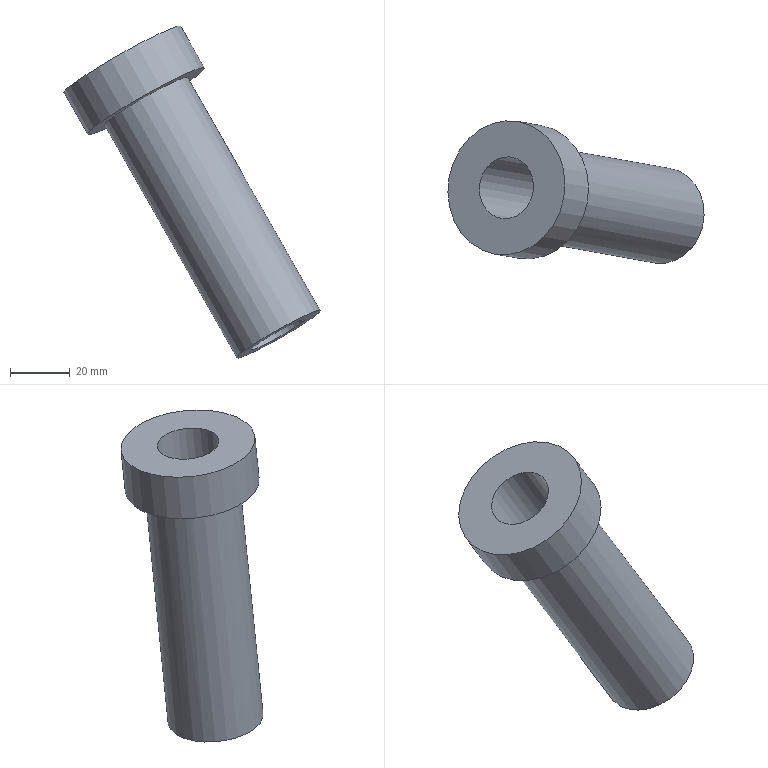Part | NX | features solid 2 | 1 solid | 6 faces | box 85.704 x 47.558 x 111.049 mm | volume 61811 mm3 | cylinder 3 | plane 3 | commonest cylinder face diameters 20.8 x1 32 x1 45 x1
STEP:
#1=CARTESIAN_POINT('',(-987.93,513.799,94.306));
#2=VERTEX_POINT('',#1);
#3=CARTESIAN_POINT('',(-996.8,515.363,89.106));
#4=DIRECTION('',(0.4924,-0.08682,-0.866));
#5=DIRECTION('',(0.8529,-0.1504,0.5));
#6=AXIS2_PLACEMENT_3D('',#3,#4,#5);
#7=CIRCLE('',#6,10.4);
#8=EDGE_CURVE('',#2,#2,#7,.T.);
#9=ORIENTED_EDGE('',*,*,#8,.F.);
#10=EDGE_LOOP('',(#9));
#11=FACE_BOUND('',#10,.T.);
#12=CARTESIAN_POINT('',(-953.646,506.16,-7.834));
#13=VERTEX_POINT('',#12);
#14=CARTESIAN_POINT('',(-944.605,506.16,-2.693));
#15=DIRECTION('',(0.4924,-0.08682,-0.866));
#16=DIRECTION('',(-0.8693,0.,-0.4943));
#17=AXIS2_PLACEMENT_3D('',#14,#15,#16);
#18=CIRCLE('',#17,10.4);
#19=EDGE_CURVE('',#13,#13,#18,.T.);
#20=ORIENTED_EDGE('',*,*,#19,.T.);
#21=EDGE_LOOP('',(#20));
#22=FACE_BOUND('',#21,.T.);
#23=CARTESIAN_POINT('',(-1026.345,520.573,141.067));
#24=DIRECTION('',(0.4924,-0.08682,-0.866));
#25=DIRECTION('',(-0.1736,-0.9848,0.));
#26=AXIS2_PLACEMENT_3D('',#23,#24,#25);
#27=CYLINDRICAL_SURFACE('',#26,10.4);
#28=ADVANCED_FACE('',(#11,#22),#27,.F.);
#29=CARTESIAN_POINT('',(-1002.568,516.38,67.249));
#30=VERTEX_POINT('',#29);
#31=CARTESIAN_POINT('',(-988.922,513.974,75.249));
#32=DIRECTION('',(-0.4924,0.08682,0.866));
#33=DIRECTION('',(-0.8529,0.1504,-0.5));
#34=AXIS2_PLACEMENT_3D('',#31,#32,#33);
#35=CIRCLE('',#34,16.);
#36=EDGE_CURVE('',#30,#30,#35,.T.);
#37=ORIENTED_EDGE('',*,*,#36,.F.);
#38=EDGE_LOOP('',(#37));
#39=FACE_BOUND('',#38,.T.);
#40=CARTESIAN_POINT('',(-958.514,506.16,-10.601));
#41=VERTEX_POINT('',#40);
#42=CARTESIAN_POINT('',(-944.605,506.16,-2.693));
#43=DIRECTION('',(0.4924,-0.08682,-0.866));
#44=DIRECTION('',(-0.8693,0.,-0.4943));
#45=AXIS2_PLACEMENT_3D('',#42,#43,#44);
#46=CIRCLE('',#45,16.);
#47=EDGE_CURVE('',#41,#41,#46,.T.);
#48=ORIENTED_EDGE('',*,*,#47,.F.);
#49=EDGE_LOOP('',(#48));
#50=FACE_BOUND('',#49,.T.);
#51=CARTESIAN_POINT('',(-1018.466,519.184,127.211));
#52=DIRECTION('',(0.4924,-0.08682,-0.866));
#53=DIRECTION('',(-0.1736,-0.9848,0.));
#54=AXIS2_PLACEMENT_3D('',#51,#52,#53);
#55=CYLINDRICAL_SURFACE('',#54,16.);
#56=ADVANCED_FACE('',(#39,#50),#55,.T.);
#57=CARTESIAN_POINT('',(-1008.111,517.358,63.999));
#58=VERTEX_POINT('',#57);
#59=CARTESIAN_POINT('',(-988.922,513.974,75.249));
#60=DIRECTION('',(-0.4924,0.08682,0.866));
#61=DIRECTION('',(-0.8529,0.1504,-0.5));
#62=AXIS2_PLACEMENT_3D('',#59,#60,#61);
#63=CIRCLE('',#62,22.5);
#64=EDGE_CURVE('',#58,#58,#63,.F.);
#65=ORIENTED_EDGE('',*,*,#64,.T.);
#66=EDGE_LOOP('',(#65));
#67=FACE_BOUND('',#66,.T.);
#68=ORIENTED_EDGE('',*,*,#36,.T.);
#69=EDGE_LOOP('',(#68));
#70=FACE_BOUND('',#69,.T.);
#71=CARTESIAN_POINT('',(-935.85,1.98,156.755));
#72=DIRECTION('',(0.4924,-0.08682,-0.866));
#73=DIRECTION('',(0.8693,0.,0.4943));
#74=AXIS2_PLACEMENT_3D('',#71,#72,#73);
#75=PLANE('',#74);
#76=ADVANCED_FACE('',(#67,#70),#75,.T.);
#77=CARTESIAN_POINT('',(-977.611,511.98,100.356));
#78=VERTEX_POINT('',#77);
#79=CARTESIAN_POINT('',(-996.8,515.363,89.106));
#80=DIRECTION('',(0.4924,-0.08682,-0.866));
#81=DIRECTION('',(0.8529,-0.1504,0.5));
#82=AXIS2_PLACEMENT_3D('',#79,#80,#81);
#83=CIRCLE('',#82,22.5);
#84=EDGE_CURVE('',#78,#78,#83,.T.);
#85=ORIENTED_EDGE('',*,*,#84,.T.);
#86=EDGE_LOOP('',(#85));
#87=FACE_BOUND('',#86,.T.);
#88=ORIENTED_EDGE('',*,*,#64,.F.);
#89=EDGE_LOOP('',(#88));
#90=FACE_BOUND('',#89,.T.);
#91=CARTESIAN_POINT('',(-1026.345,520.573,141.067));
#92=DIRECTION('',(0.4924,-0.08682,-0.866));
#93=DIRECTION('',(-0.1736,-0.9848,0.));
#94=AXIS2_PLACEMENT_3D('',#91,#92,#93);
#95=CYLINDRICAL_SURFACE('',#94,22.5);
#96=ADVANCED_FACE('',(#87,#90),#95,.T.);
#97=ORIENTED_EDGE('',*,*,#84,.F.);
#98=EDGE_LOOP('',(#97));
#99=FACE_BOUND('',#98,.T.);
#100=ORIENTED_EDGE('',*,*,#8,.T.);
#101=EDGE_LOOP('',(#100));
#102=FACE_BOUND('',#101,.T.);
#103=CARTESIAN_POINT('',(-996.8,515.363,89.106));
#104=DIRECTION('',(-0.4924,0.08682,0.866));
#105=DIRECTION('',(0.1736,0.9848,0.));
#106=AXIS2_PLACEMENT_3D('',#103,#104,#105);
#107=PLANE('',#106);
#108=ADVANCED_FACE('',(#99,#102),#107,.T.);
#109=ORIENTED_EDGE('',*,*,#19,.F.);
#110=EDGE_LOOP('',(#109));
#111=FACE_BOUND('',#110,.T.);
#112=ORIENTED_EDGE('',*,*,#47,.T.);
#113=EDGE_LOOP('',(#112));
#114=FACE_BOUND('',#113,.T.);
#115=CARTESIAN_POINT('',(-970.389,-107.759,44.196));
#116=DIRECTION('',(0.4924,-0.08682,-0.866));
#117=DIRECTION('',(-0.8693,0.,-0.4943));
#118=AXIS2_PLACEMENT_3D('',#115,#116,#117);
#119=PLANE('',#118);
#120=ADVANCED_FACE('',(#111,#114),#119,.T.);
#121=CLOSED_SHELL('',(#28,#56,#76,#96,#108,#120));
#122=MANIFOLD_SOLID_BREP('',#121);
#123=(LENGTH_UNIT()NAMED_UNIT(*)SI_UNIT(.MILLI.,.METRE.));
#124=UNCERTAINTY_MEASURE_WITH_UNIT(LENGTH_MEASURE(0.00001),#123,'','');
#125=(NAMED_UNIT(*)PLANE_ANGLE_UNIT()SI_UNIT($,.RADIAN.));
#126=(NAMED_UNIT(*)SI_UNIT($,.STERADIAN.)SOLID_ANGLE_UNIT());
#127=(GEOMETRIC_REPRESENTATION_CONTEXT(3)GLOBAL_UNCERTAINTY_ASSIGNED_CONTEXT((#124))GLOBAL_UNIT_ASSIGNED_CONTEXT((#123,#125,#126))REPRESENTATION_CONTEXT('',''));
#128=ADVANCED_BREP_SHAPE_REPRESENTATION('',(#122),#127);